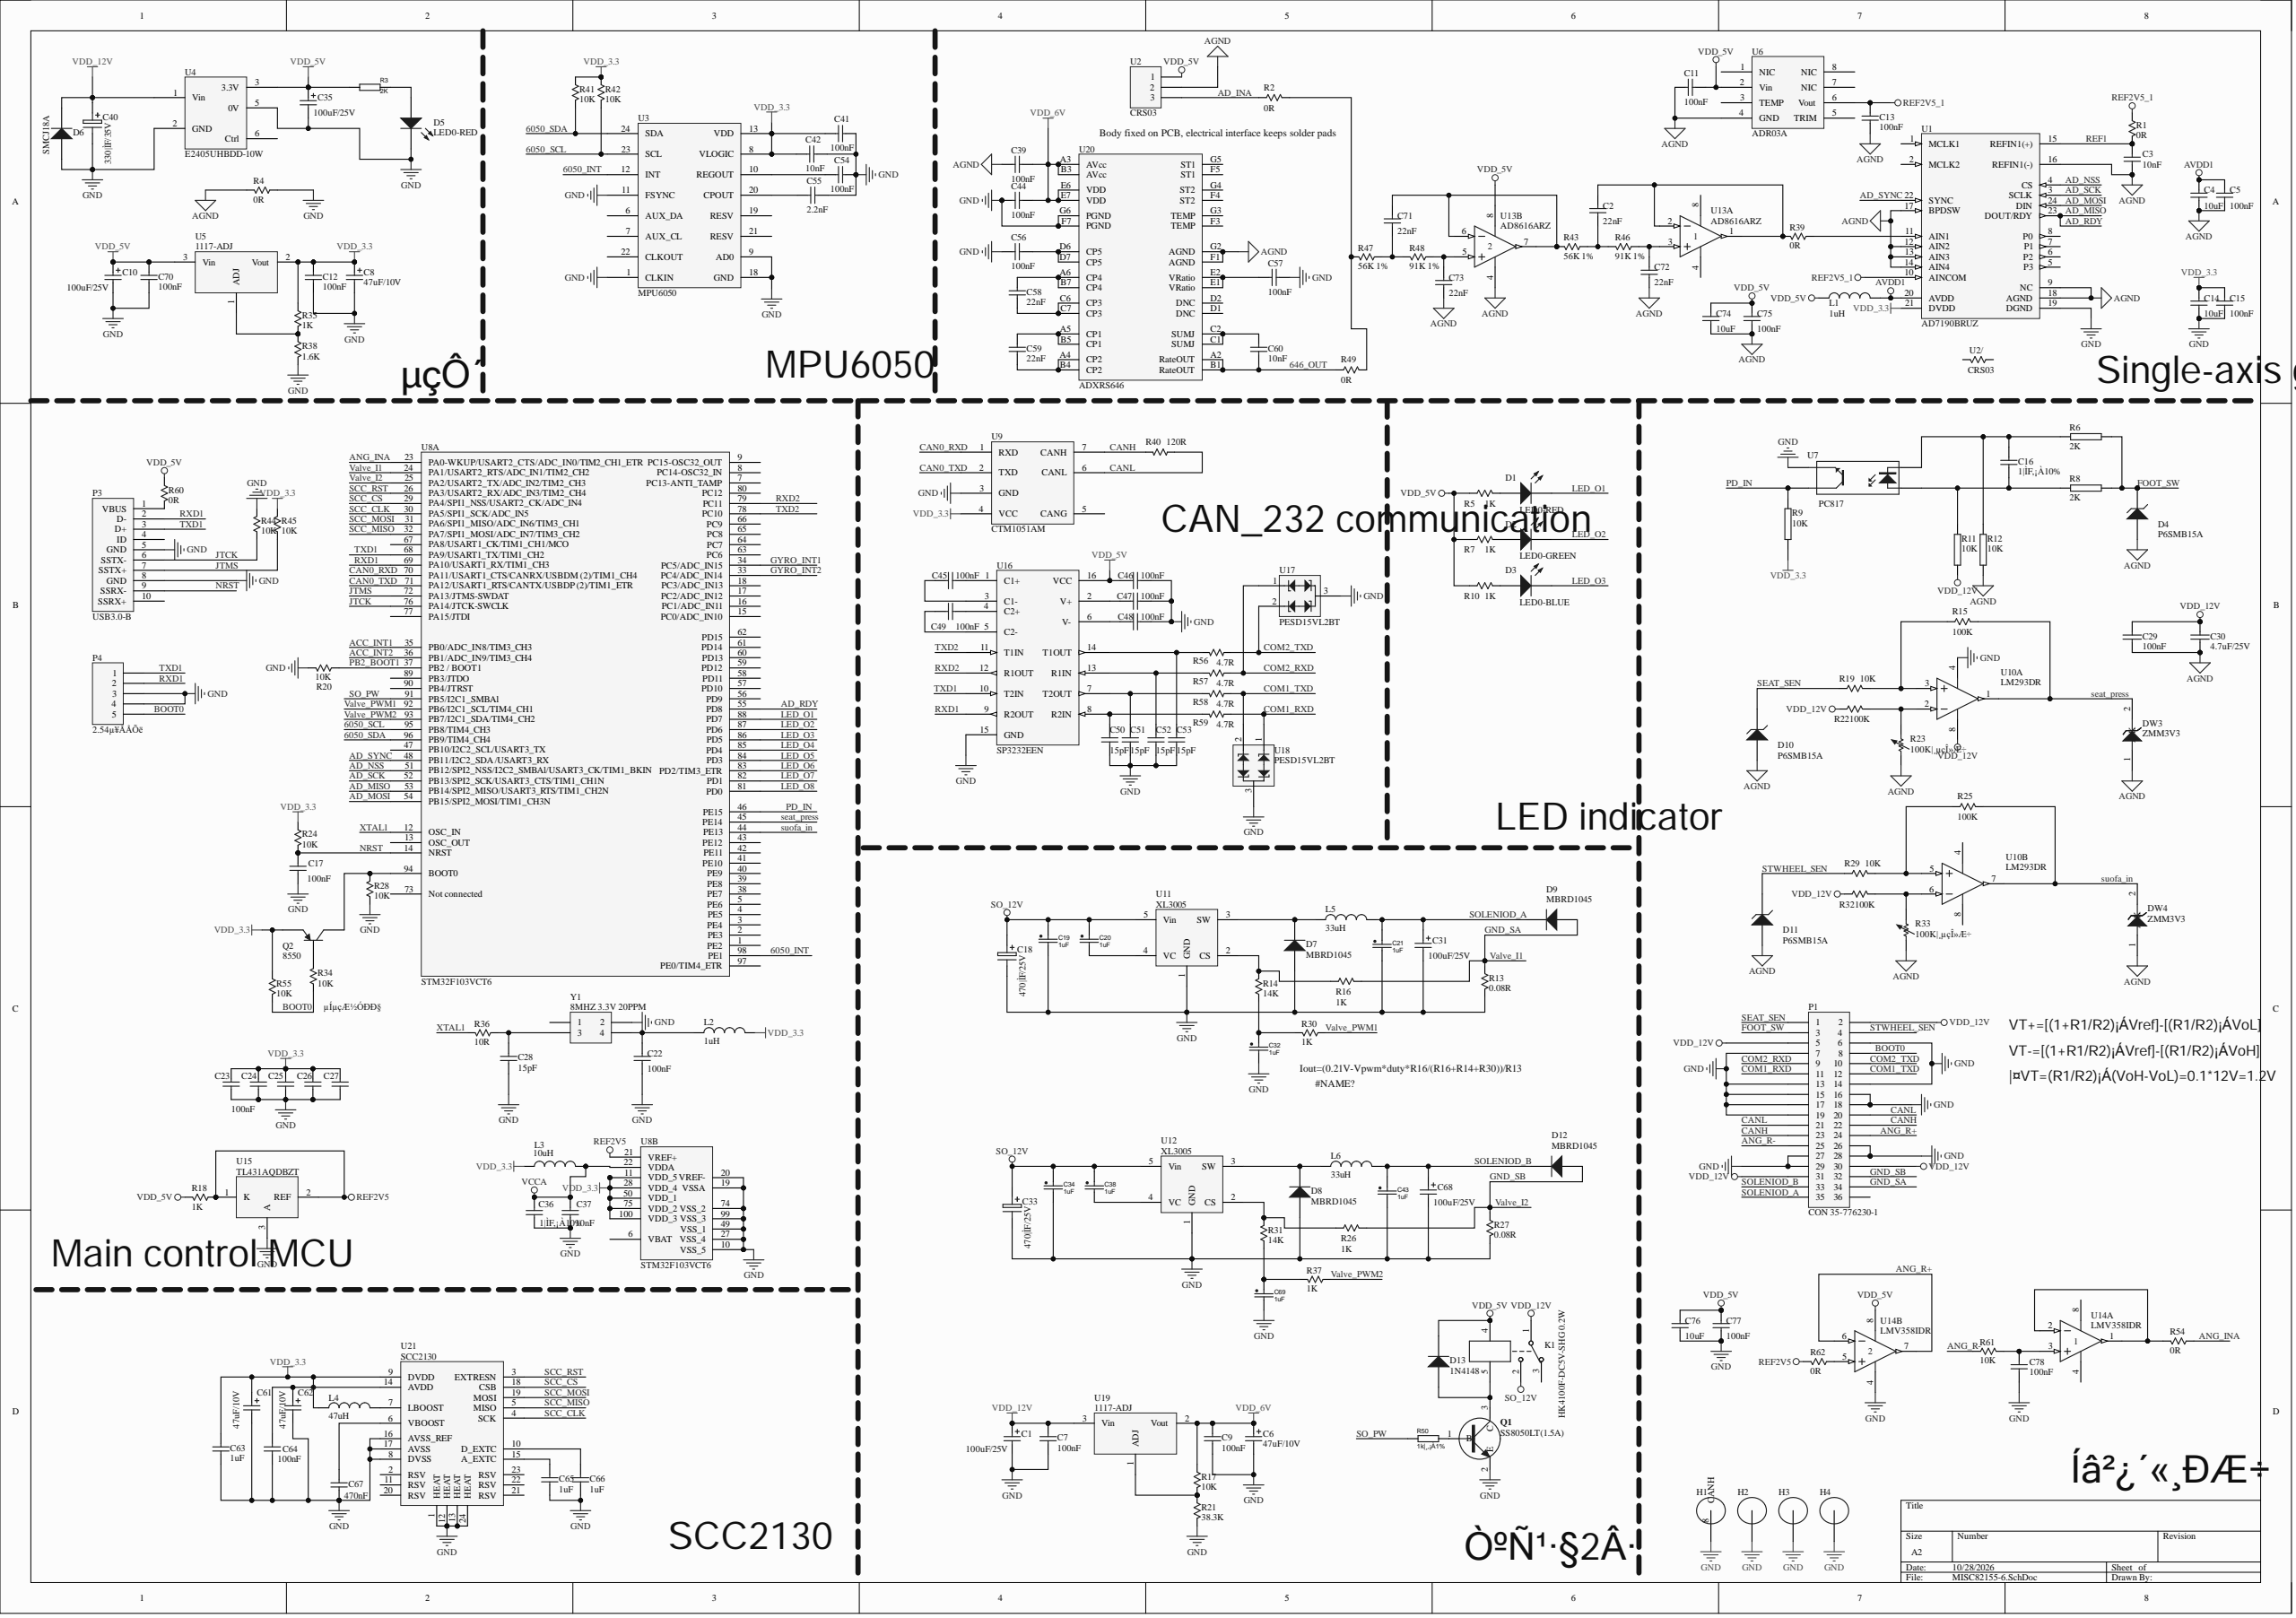Circuit board | Altium Designer | 191 parts | 125 nets
Bill of materials:
Comment,Description,Designator,Footprint,LibRef,Quantity
"100uF/25V","Polarized Capacitor (Axial)","C1, C10, C31, C35, C68","RB6.3*7","Cap Pol2","5"
"22nF","Capacitor","C2, C58, C59, C71, C72, C73","C0805","Cap","6"
"10nF","Capacitor","C3, C37, C42, C60","C0805","Cap","4"
"10uF","Capacitor","C4, C14, C74, C76","C0805","Cap","4"
"100nF","Capacitor","C5, C7, C9, C11, C12, C13, C15, C17, C22, C23, C24, C25, C26, C27, C29, C39, C41, C44, C45, C46, C47, C48, C49, C54, C56, C57, C64, C70, C75, C77, C78","C0805","Cap","31"
"47uF/10V","Polarized Capacitor (Axial)","C6, C8, C61, C62","CT3528-B","Cap Pol2","4"
"1|ÌF,¡À10%","Capacitor","C16, C36","C0805","Cap","2"
"470|ÌF/25V","220|ÌF,16V,§¶6.3¡Á7mm,,珠海华冠,RoHS","C18, C33","CAPPR5.0-10X16-0.8","1.02.11.0018","2"
"1uF","[NoValue], Capacitor","C19, C20, C21, C32, C34, C38, C43, C63, C65, C66, C69","C0805","CAP NP_Dup5, Cap","11"
"15pF","Capacitor","C28, C50, C51, C52, C53","C0805","Cap","5"
"4.7uF/25V","Capacitor","C30","1206C","CAP","1"
"330|ÌF/35V","220|ÌF,16V,§¶6.3¡Á7mm,,珠海华冠,RoHS","C40","CAPPR5.0-10X16-0.8","1.02.11.0018","1"
"2.2nF","Capacitor","C55","C0805","Cap","1"
"470nF","Capacitor","C67","C0805","Cap","1"
"LED0-RED","Typical INFRARED GaAs LED","D1, D5","LED0805","LED0","2"
"LED0-GREEN","Typical INFRARED GaAs LED","D2","LED0805","LED0","1"
"LED0-BLUE","Typical INFRARED GaAs LED","D3","LED0805","LED0","1"
"P6SMB15A","Zener Diode","D4, D10, D11","DO-214","D Zener","3"
"SMCJ18A","1 Amp General Purpose Rectifier","D6","SMC","Diode 1N4007","1"
"MBRD1045","1 Amp General Purpose Rectifier","D7, D8, D9, D12","TO-252","Diode 1N4007","4"
"1N4148","Default Diode","D13","SMD-D4148","Diode","1"
"ZMM3V3","Zener Diode","DW3, DW4","SMD-D4148","ZENER3","2"
"Hole","Hole","H1, H2, H3, H4","HOLE-3.2","Hole","4"
"HK4100F-DC5V-SHG 0.2W","Single-Pole Dual-Throw Relay","K1","HK4100F","Relay-SPDT","1"
"1uH","Inductor","L1, L2","R0805","Inductor","2"
"10uH","Inductor","L3","R0805","Inductor","1"
"47uH","Inductor","L4","R1210","Inductor","1"
"33uH","Inductor","L5, L6","SLF12555","Inductor","2"
"CON 35-776230-1","Header, 18-Pin, Dual row","P1","VGA35","Header 18X2","1"
"USB3.0-B","","P3","Micro USB3.0-B","USB3.0-B","1"
"2.54单排针","Header, 5-Pin","P4","HDR1X5","Header 5","1"
"SS8050LT(1.5A)","SS8050LT(1.5A),SOT-23,Jiangsu Changdian,RoHS","Q1","SOT-23","1.04.09.0001","1"
"8550","PNP Bipolar Transistor","Q2","SOT-23","PNP","1"
"0R","Resistor","R1, R2, R4, R39, R49, R54, R60, R62","R0805","Res","8"
"2K","","R3, R6, R8","R0805","RES, 1.01.17.0004","3"
"1K","Resistor","R5, R7, R10, R16, R18, R26, R30, R35, R37","R0805","Res","9"
"10K","[NoValue], Resistor","R9, R11, R12, R17, R19, R20, R24, R28, R29, R34, R41, R42, R44, R45, R55, R61","R0805","1.01.17.0004, Res","16"
"0.08R","Resistor","R13, R27","R2512","Res","2"
"14K","Resistor","R14, R31","R0805","Res","2"
"100K","Resistor","R15, R22, R25, R32","R0805","Res","4"
"38.3K","Resistor","R21","R0805","Res","1"
"100K|¸µçÎ»Æ÷","Variable Resistor","R23, R33","CHANGER3","Res Adj1","2"
"10R","Resistor","R36","R0805","Res","1"
"1.6K","Resistor","R38","R0805","Res","1"
"120R","Resistor","R40","R0805","Res","1"
"56K 1%","Resistor","R43, R47","R0805","Res","2"
"91K 1%","Resistor","R46, R48","R0805","Res","2"
"1k|¸,¡À1%","","R50","0805R","RES","1"
"4.7R","Resistor","R56, R57, R58, R59","R0805","Res","4"
"AD7190BRUZ","","U1","IC-24P-TSSOP-6_4MM-G","AD7190","1"
"CRS03","Header, 3-Pin","U2","HDR1X3","Header 3","1"
"CRS03","Resistor","U2/","CDS43-01","Res","1"
"MPU6050","3-axi gyros","U3","QFN24","ITG3050","1"
"E2405UHBDD-10W","","U4","E2403UHBDD","E2403UHBDD-10W","1"
"1117-ADJ","","U5, U19","SOT-223","VOLTREG1","2"
"ADR03A","","U6","SOP-8","ADR03ARZ","1"
"PC817","Optoisolator","U7","SMD-4","TLP281-1","1"
"STM32F103VCT6","","U8","QFP-100","STM32F103VBH6","1"
"CTM1051AM","CTM1051AM","U9","CTM1051AM","CTM1051AM","1"
"LM293DR","Dual Comparator","U10","SOP-8","LM293D","1"
"XL3005","XL3005","U11, U12","TO-263-5","XL3005","2"
"AD8616ARZ","Dual Low-Power Operational Amplifier","U13","SOP-8","LM358D","1"
"LMV358IDR","Dual Low-Power Operational Amplifier","U14","SOP-8","LM358D","1"
"TL431AQDBZT","TL431A","U15","LC-SOT-23(SOT-23-3)","TL431A","1"
"SP3232EEN","","U16","SOP16-6.6","SP202ECT","1"
"PESD15VL2BT","","U17, U18","SOT-23","PESD12VL2BT","2"
"ADXRS646","ADXRS646","U20","","ADXRS646","1"
"SCC2130","","U21","SCC2130D","SCC2130","1"
"8MHZ 3.3V 20PPM","Header, 2-Pin, Dual row","Y1","XTAL7050","Header 2X2","1"
Netlist (Protel format):
[
C1
RB6.3*7
100uF/25V



]
[
C2
C0805
22nF



]
[
C3
C0805
10nF



]
[
C4
C0805
10uF



]
[
C5
C0805
100nF



]
[
C6
CT3528-B
47uF/10V



]
[
C7
C0805
100nF



]
[
C8
CT3528-B
47uF/10V



]
[
C9
C0805
100nF



]
[
C10
RB6.3*7
100uF/25V



]
[
C11
C0805
100nF



]
[
C12
C0805
100nF



]
[
C13
C0805
100nF



]
[
C14
C0805
10uF



]
[
C15
C0805
100nF



]
[
C16
C0805
1|ÌF,¡À10%



]
[
C17
C0805
100nF



]
[
C18
CAPPR5.0-10X16-0.8
470|ÌF/25V



]
[
C19
C0805
1uF



]
[
C20
C0805
1uF



]
[
C21
C0805
1uF



]
[
C22
C0805
100nF



]
[
C23
C0805
100nF



]
[
C24
C0805
100nF



]
[
C25
C0805
100nF



]
[
C26
C0805
100nF



]
[
C27
C0805
100nF



]
[
C28
C0805
15pF



]
[
C29
C0805
100nF



]
[
C30
1206C
4.7uF/25V



]
[
C31
RB6.3*7
100uF/25V



]
[
C32
C0805
1uF



]
[
C33
CAPPR5.0-10X16-0.8
470|ÌF/25V



]
[
C34
C0805
1uF



]
[
C35
RB6.3*7
100uF/25V



]
[
C36
C0805
1|ÌF,¡À10%



]
[
C37
C0805
10nF



]
[
C38
C0805
1uF



]
[
C39
C0805
100nF



]
[
C40
CAPPR5.0-10X16-0.8
330|ÌF/35V



]
[
C41
C0805
100nF



]
[
C42
C0805
10nF



]
[
C43
C0805
1uF



]
[
C44
C0805
100nF



]
[
C45
C0805
100nF



]
[
C46
C0805
100nF



]
[
C47
C0805
100nF



]
[
C48
C0805
100nF



]
[
C49
C0805
100nF



]
[
C50
C0805
15pF



]
[
C51
C0805
15pF



]
[
C52
C0805
15pF



]
[
C53
C0805
15pF



]
[
C54
C0805
100nF



]
[
C55
C0805
2.2nF



]
[
C56
C0805
100nF



]
[
C57
C0805
100nF



]
[
C58
C0805
22nF



]
[
C59
C0805
22nF



]
[
C60
C0805
10nF



]
[
C61
CT3528-B
47uF/10V



]
[
C62
CT3528-B
47uF/10V



]
[
C63
C0805
1uF



]
[
C64
C0805
100nF



]
[
C65
C0805
1uF



]
[
C66
C0805
1uF



]
[
C67
C0805
470nF



]
[
C68
RB6.3*7
100uF/25V



]
[
C69
C0805
1uF



]
[
C70
C0805
100nF



]
[
C71
C0805
22nF



]
[
C72
C0805
22nF



]
[
C73
C0805
22nF



]
[
C74
C0805
10uF



]
[
C75
C0805
100nF



]
[
C76
C0805
10uF



]
[
C77
C0805
100nF



]
[
C78
C0805
100nF



]
[
D1
LED0805
LED0-RED



]
[
D2
LED0805
LED0-GREEN



]
[
D3
LED0805
LED0-BLUE



]
[
D4
DO-214
P6SMB15A



]
[
D5
LED0805
LED0-RED



]
[
D6
SMC
SMCJ18A



]
[
D7
TO-252
MBRD1045



]
[
D8
TO-252
MBRD1045



]
[
D9
TO-252
MBRD1045



]
[
D10
DO-214
P6SMB15A



]
[
D11
DO-214
P6SMB15A



]
[
D12
TO-252
MBRD1045



]
[
D13
SMD-D4148
1N4148



]
[
DW3
SMD-D4148
ZMM3V3



]
[
DW4
SMD-D4148
ZMM3V3



]
[
H1
HOLE-3.2
Hole



]
[
H2
HOLE-3.2
Hole



]
[
H3
HOLE-3.2
Hole



]
[
H4
HOLE-3.2
Hole



]
[
K1
HK4100F
HK4100F-DC5V-SHG 0.2W



]
[
L1
R0805
1uH



]
[
L2
R0805
1uH



]
[
L3
R0805
10uH



]
[
L4
R1210
47uH



]
[
L5
SLF12555
33uH



]
[
L6
SLF12555
33uH



]
[
P1
VGA35
CON 35-776230-1



]
[
P3
Micro USB3.0-B
USB3.0-B



]
[
P4
HDR1X5
2.54单排针



]
[
Q1
SOT-23
SS8050LT(1.5A)



]
[
Q2
SOT-23
8550



]
[
R1
R0805
0R



]
[
R2
R0805
0R



]
[
R3
R0805
2K



]
[
R4
R0805
0R



]
[
R5
R0805
1K



]
[
R6
R0805
2K



]
[
R7
R0805
1K



]
[
R8
R0805
2K



]
[
R9
R0805
10K



]
[
R10
R0805
1K



]
[
R11
R0805
10K



]
[
R12
R0805
10K



]
[
R13
R2512
0.08R



]
[
R14
R0805
14K



]
[
R15
R0805
100K



]
[
R16
R0805
1K



]
[
R17
R0805
10K



]
[
R18
R0805
1K



]
[
R19
R0805
10K



]
[
R20
R0805
10K



]
[
R21
R0805
38.3K



]
[
R22
R0805
100K



]
[
R23
CHANGER3
100K|¸µçÎ»Æ÷



]
[
R24
R0805
10K



]
[
R25
R0805
100K



]
[
R26
R0805
1K



]
[
R27
R2512
0.08R



]
[
R28
R0805
10K



]
[
R29
R0805
10K



]
[
R30
R0805
1K



]
[
R31
R0805
14K



]
[
R32
R0805
100K



]
[
R33
CHANGER3
100K|¸µçÎ»Æ÷



]
[
R34
R0805
10K



]
[
R35
R0805
1K



]
[
R36
R0805
10R



]
[
R37
R0805
1K



]
[
R38
R0805
1.6K



]
[
R39
R0805
0R



]
[
R40
R0805
120R



]
[
R41
R0805
10K



]
[
R42
R0805
10K



]
[
R43
R0805
56K 1%



]
[
R44
R0805
10K



]
[
R45
R0805
10K



]
[
R46
R0805
91K 1%



]
[
R47
R0805
56K 1%



]
[
R48
R0805
91K 1%



]
[
R49
R0805
0R



]
[
R50
0805R
1k|¸,¡À1%



]
[
R54
R0805
0R



]
[
R55
R0805
10K



]
[
R56
R0805
4.7R



]
[
R57
R0805
4.7R



]
[
R58
R0805
4.7R



]
[
R59
R0805
4.7R



]
[
R60
R0805
0R



]
[
R61
R0805
10K



]
[
R62
R0805
0R



]
[
U1
IC-24P-TSSOP-6_4MM-G
AD7190BRUZ



]
[
U2
HDR1X3
CRS03



]
[
U2/
CDS43-01
CRS03



]
[
U3
QFN24
MPU6050



]
[
U4
E2403UHBDD
E2405UHBDD-10W



]
[
U5
SOT-223
1117-ADJ



]
[
U6
SOP-8
ADR03A



]
[
U7
SMD-4
PC817



]
[
U8
QFP-100
STM32F103VCT6



]
[
U9
CTM1051AM
CTM1051AM



]
[
U10
SOP-8
LM293DR



]
[
U11
TO-263-5
XL3005



]
[
U12
TO-263-5
XL3005



]
[
U13
SOP-8
AD8616ARZ



]
[
U14
SOP-8
LMV358IDR



]
[
U15
LC-SOT-23(SOT-23-3)
TL431AQDBZT



]
[
U16
SOP16-6.6
SP3232EEN



]
[
U17
SOT-23
PESD15VL2BT



]
[
U18
SOT-23
PESD15VL2BT



]
[
U19
SOT-223
1117-ADJ



]
[
U20

ADXRS646



]
[
U21
SCC2130D
SCC2130



]
[
Y1
XTAL7050
8MHZ 3.3V 20PPM



]
(
XTAL1
R36-1
U8-12
)
(
VDD_12V
C1-1
C7-2
C29-1
C30-1
C40-1
D6-2
K1-1
P1-2
P1-5
P1-30
P1-31
R11-2
R22-2
R32-2
U4-1
U10-8
U19-3
)
(
VDD_6V
C6-1
C9-2
C39-2
C44-2
R17-2
U19-2
U20-A3
U20-B3
U20-E6
U20-E7
)
(
VDD_5V
C10-1
C11-2
C35-1
C46-1
C70-2
C74-1
C75-1
C76-1
C77-1
D13-2
K1-4
L1-1
R3-2
R5-2
R7-2
R10-2
R18-1
R60-1
U2-1
U4-3
U5-3
U6-2
U13-8
U14-8
U16-16
)
(
VDD_3.3
C8-1
C12-2
C14-1
C15-1
C23-1
C24-1
C25-1
C26-1
C27-1
C41-2
C42-2
C61-1
C62-1
C63-1
C64-1
L2-2
L3-1
L4-1
Q2-2
R9-1
R24-2
R35-2
R41-2
R42-2
R45-1
R55-2
U1-21
U3-8
U3-13
U5-2
U8-11
U8-28
U8-50
U8-75
U8-100
U9-4
U21-9
U21-14
)
(
VCCA
C36-2
C37-2
L3-2
U8-22
)
(
Valve_PWM2
R37-1
U8-93
)
(
Valve_PWM1
R30-1
U8-92
)
(
TXD2
U8-78
U16-11
)
(
TXD1
P3-3
P4-1
U8-68
U16-10
)
(
suofa_in
DW4-2
R25-1
U8-44
U10-7
)
(
STWHEEL_SEN
D11-2
P1-4
R29-2
)
(
SOLENIOD_B
C43-1
C68-1
D12-2
L6-2
P1-33
)
(
SOLENIOD_A
C21-1
C31-1
D9-2
L5-2
P1-35
)
(
SO_PW
R50-1
U8-91
)
(
SO_12V
C18-1
C19-1
C20-1
C33-1
C34-1
C38-1
K1-2
U11-5
U12-5
)
(
SEAT_SEN
D10-2
P1-1
R19-2
)
(
seat_press
DW3-2
R15-1
U8-45
U10-1
)
(
SCC_RST
U8-26
U21-3
)
(
SCC_MOSI
U8-31
U21-19
)
(
SCC_MISO
U8-32
U21-5
)
(
SCC_CS
U8-29
U21-18
)
(
SCC_CLK
U8-30
U21-4
)
(
RXD2
U8-79
U16-12
)
(
RXD1
P3-2
P4-2
U8-69
U16-9
)
(
REF2V5_1
C13-1
R1-2
U1-10
U6-6
)
(
REF2V5
R18-2
R62-1
U8-21
U15-1
U15-2
)
(
REF1
C3-1
R1-1
U1-15
)
(
PD_IN
R9-2
U7-4
U8-46
)
(
PB2_BOOT1
R20-2
U8-37
)
(
NRST
C17-2
P3-9
R24-1
U8-14
)
(
NetR62_2
R62-2
U14-5
)
(
NetR54_1
R54-1
U14-1
U14-2
)
(
NetR39_2
R39-2
U1-11
)
(
NetR35_1
R35-1
R38-2
U5-1
)
(
NetR32_1
R32-1
R33-2
U10-6
)
(
NetR26_2
R26-2
R31-1
U12-2
)
(
NetR25_2
R25-2
R29-1
U10-5
)
(
NetR22_1
R22-1
R23-2
U10-2
)
(
NetR17_1
R17-1
R21-2
U19-1
)
(
NetR15_2
R15-2
R19-1
U10-3
)
(
NetR14_1
R14-1
R16-2
U11-2
)
(
NetR2_1
R2-1
R47-1
R49-1
)
(
NetQ2_3
Q2-3
R28-2
U8-94
)
(
NetQ2_1
Q2-1
R34-1
)
(
NetQ1_1
Q1-1
R50-2
)
(
NetP3_1
P3-1
R60-2
)
(
NetL4_2
L4-2
U21-7
)
(
NetD13_1
D13-1
K1-5
Q1-3
)
(
NetD8_2
D8-2
L6-1
U12-3
)
(
NetD7_2
D7-2
L5-1
U11-3
)
(
NetD5_1
D5-1
R3-1
)
(
NetD3_1
D3-1
R10-1
)
(
NetD2_1
D2-1
R7-1
)
(
NetD1_1
D1-1
R5-1
)
(
NetC78_1
C78-1
R61-1
U14-3
)
(
NetC73_1
C73-1
R48-2
U13-5
)
(
NetC72_1
C72-1
R46-2
U13-3
)
(
NetC71_2
C71-2
R47-2
R48-1
)
(
NetC71_1
C71-1
R43-1
U13-6
U13-7
)
(
NetC69_1
C69-1
R31-2
R37-2
)
(
NetC67_1
C67-1
U21-6
)
(
NetC66_1
C66-1
U21-10
)
(
NetC65_1
C65-1
U21-15
)
(
NetC60_2
C60-2
U20-C1
U20-C2
)
(
NetC59_2
C59-2
U20-A4
U20-B4
)
(
NetC59_1
C59-1
U20-A5
U20-B5
)
(
NetC58_2
C58-2
U20-C6
U20-C7
)
(
NetC58_1
C58-1
U20-A6
U20-B7
)
(
NetC57_1
C57-1
U20-E1
U20-E2
)
(
NetC56_2
C56-2
U20-D6
U20-D7
)
(
NetC55_2
C55-2
U3-20
)
(
NetC54_2
C54-2
U3-10
)
(
NetC53_1
C53-1
R56-1
U16-14
)
(
NetC52_1
C52-1
R57-1
U16-13
)
(
NetC51_1
C51-1
R58-1
U16-7
)
(
NetC50_1
C50-1
R59-1
U16-8
)
(
NetC49_2
C49-2
U16-4
)
(
NetC49_1
C49-1
U16-5
)
(
NetC48_1
C48-1
U16-6
)
(
NetC47_1
C47-1
U16-2
)
(
NetC45_2
C45-2
U16-1
)
(
NetC45_1
C45-1
U16-3
)
(
NetC38_2
C38-2
U12-4
)
(
NetC32_1
C32-1
R14-2
R30-2
)
(
NetC28_2
C28-2
R36-2
Y1-3
)
(
NetC22_1
C22-1
L2-1
Y1-4
)
(
NetC20_2
C20-2
U11-4
)
(
NetC16_2
C16-2
R6-2
R12-1
U7-2
)
(
NetC16_1
C16-1
R8-2
R11-1
U7-1
)
(
NetC2_2
C2-2
R43-2
R46-1
)
(
NetC2_1
C2-1
R39-1
U13-1
U13-2
)
(
LED_O3
D3-2
U8-86
)
(
LED_O2
D2-2
U8-87
)
(
LED_O1
D1-2
U8-88
)
(
JTMS
P3-7
R45-2
U8-72
)
(
JTCK
P3-6
R44-2
U8-76
)
(
GND_SB
D12-1
P1-32
R26-1
R27-2
U8-25
)
(
GND_SA
D9-1
P1-34
R13-2
R16-1
U8-24
)
(
GND
C1-2
C6-2
C7-1
C8-2
C9-1
C10-2
C12-1
C14-2
C15-2
C17-1
C18-2
C19-2
C21-2
C22-2
C23-2
C24-2
C25-2
C26-2
C27-2
C28-1
C31-2
C32-2
C33-2
C34-2
C35-2
C36-1
C37-1
C40-2
C41-1
C42-1
C43-2
C44-1
C46-2
C47-2
C48-2
C50-2
C51-2
C52-2
C53-2
C54-1
C55-1
C56-1
C57-2
C61-2
C62-2
C63-2
C64-2
C65-2
C66-2
C67-2
C68-2
C69-2
C70-1
C76-2
C77-2
C78-2
D5-2
D6-1
D7-1
D8-1
H1-8
H2-8
H3-8
H4-8
P1-6
P1-7
P1-13
P1-14
P1-15
P1-16
P1-17
P1-18
P1-19
P1-26
P1-27
P1-28
P1-29
P3-5
P3-8
P4-3
P4-4
Q1-2
R4-2
R13-1
R20-1
R21-1
R27-1
R28-1
R38-1
R44-1
U1-19
U3-1
U3-9
U3-11
U3-18
U4-2
U4-5
U7-3
U8-10
U8-19
U8-20
U8-27
U8-49
U8-74
U8-99
U9-3
U10-4
U11-1
U12-1
U14-4
U15-3
U16-15
U17-3
U18-3
U20-F7
U20-G6
U21-1
U21-8
U21-12
U21-13
U21-16
U21-17
U21-24
Y1-2
)
(
FOOT_SW
D4-2
P1-3
R6-1
R8-1
)
(
COM2_TXD
P1-10
R56-2
U17-2
)
(
COM2_RXD
P1-9
R57-2
U17-1
)
(
COM1_TXD
P1-12
R58-2
U18-2
)
(
COM1_RXD
P1-11
R59-2
U18-1
)
(
CANL
P1-20
P1-21
R40-2
U9-6
)
(
CANH
P1-22
P1-23
R40-1
U9-7
)
(
CAN0_TXD
U8-71
U9-2
)
(
CAN0_RXD
U8-70
U9-1
)
(
BOOT0
P1-8
P4-5
R34-2
R55-1
)
(
AVDD1
C4-1
C5-1
L1-2
U1-20
)
(
ANG_R-
P1-25
R61-2
)
(
ANG_R+
P1-24
U14-6
U14-7
)
(
ANG_INA
R54-2
U8-23
)
(
AGND
C3-2
C4-2
C5-2
C11-1
C13-2
C29-2
C30-2
C39-1
C72-2
C73-2
C74-2
C75-2
D4-1
D10-1
D11-1
DW3-1
DW4-1
R4-1
R12-2
R23-1
R33-1
U1-9
U1-12
U1-13
U1-14
U1-16
U1-17
U1-18
U2-2
U6-4
U13-4
U20-F1
U20-G2
)
(
AD_SYNC
U1-22
U8-48
)
(
AD_SCK
U1-3
U8-52
)
(
AD_NSS
U1-4
U8-51
)
(
AD_MOSI
U1-24
U8-54
)
(
AD_MISO
U1-23
U8-53
U8-55
)
(
AD_INA
R2-2
U2-3
)
(
6050_SDA
R41-1
U3-24
U8-96
)
(
6050_SCL
R42-1
U3-23
U8-95
)
(
6050_INT
U3-12
U8-98
)
(
646_OUT
C60-1
R49-2
U20-A2
U20-B1
)